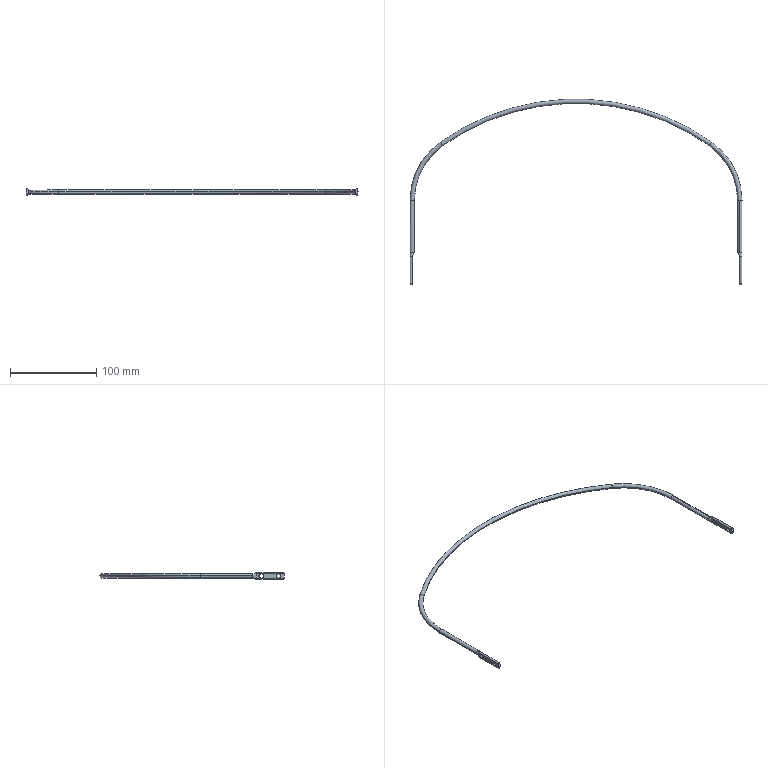Part | SolidWorks | features BaseBody 1 | 1 solid | 34 faces | box 384 x 214.497 x 8 mm | volume 13043 mm3 | cylinder 20 | torus 6 | spline 4 | plane 4 | commonest cylinder face diameters 5.2 x8 2.5 x6 5 x4 14 x2